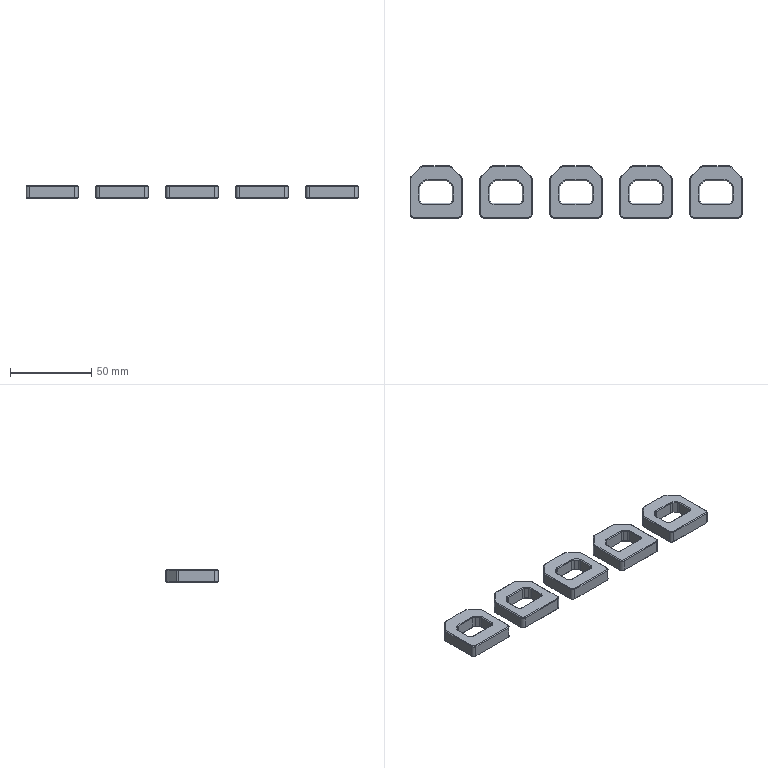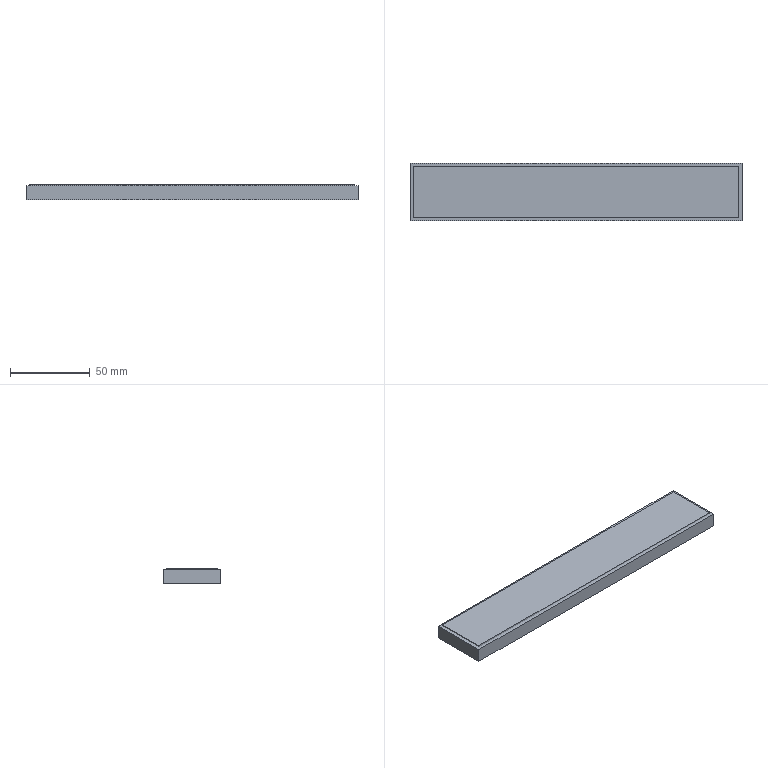CAM job | NX | 3-axis milling | part box 204 x 32 x 8 mm | stock box 208 x 36 x 10 mm
Tools:
number,name,description,diameter,corner_radius,flute_length,length,flutes
19,D80,Milling Tool-5 Parameters,80.0,0.0,50.0,75.0,2
15,D10,Milling Tool-5 Parameters,10.0,0.0,50.0,75.0,2
14,D10JING,Milling Tool-5 Parameters,10.0,0.0,50.0,75.0,2
11,D4,Milling Tool-5 Parameters,4.0,0.0,50.0,75.0,2
17,D3,Milling Tool-5 Parameters,3.0,0.0,50.0,75.0,2
1,D6A45,Milling Tool-5 Parameters,6.0,0.0,50.0,75.0,2
Operations:
program,operation,operation_type,tool,method,geometry_group,spindle_rpm,surface_speed,feed_per_tooth,feed_cut,feed_plunge,cut_length_mm,path_length_mm,cut_time_min,machine_time_min
1,FLOOR_WALL,VolumeBased25DMillingOperation,D80,METHOD,A,6500.0,1633.0,0.1154,1500.0,100.0,300.0,354.0,0.2,0.2054
1,ZLEVEL_PROFILE_COPY_1,ZLevelMilling,D10,METHOD,A,9500.0,298.0,0.1842,3500.0,1000.0,8456.651,10201.146,2.757,2.932
1,ZLEVEL_PROFILE_COPY_1_COPY,ZLevelMilling,D10JING,METHOD,A,9500.0,298.0,0.0632,1200.0,1000.0,937.046,2448.583,0.7851,0.9363
1,ZLEVEL_PROFILE_COPY_1_COPY_1,ZLevelMilling,D4,METHOD,A,9500.0,298.0,0.0947,1800.0,1000.0,2849.534,7056.004,1.756,2.177
1,HOLE_MILLING,CylinderMilling,D3,METHOD,A,9500.0,89.0,0.0605,1150.0,100.0,1388.751,3109.339,1.208,1.38
1,PLANAR_MILL_COPY_COPY_COPY_COPY,PlanarMilling,D6A45,METHOD,A,9500.0,179.0,0.0658,1250.0,100.0,1179.306,3489.985,0.9434,1.175
1,刀补17,CylinderMilling,D3,METHOD,A,9500.0,89.0,0.0605,1150.0,100.0,309.636,2030.225,0.2692,0.4413
2,FLOOR_WALL_COPY,VolumeBased25DMillingOperation,D80,METHOD,B,6500.0,1633.0,0.1154,1500.0,100.0,1200.0,2292.001,0.8,0.9092
2,PLANAR_MILL_COPY_COPY_COPY_COPY_COPY,PlanarMilling,D6A45,METHOD,B,9500.0,179.0,0.0658,1250.0,100.0,951.755,1783.755,0.7614,0.8446